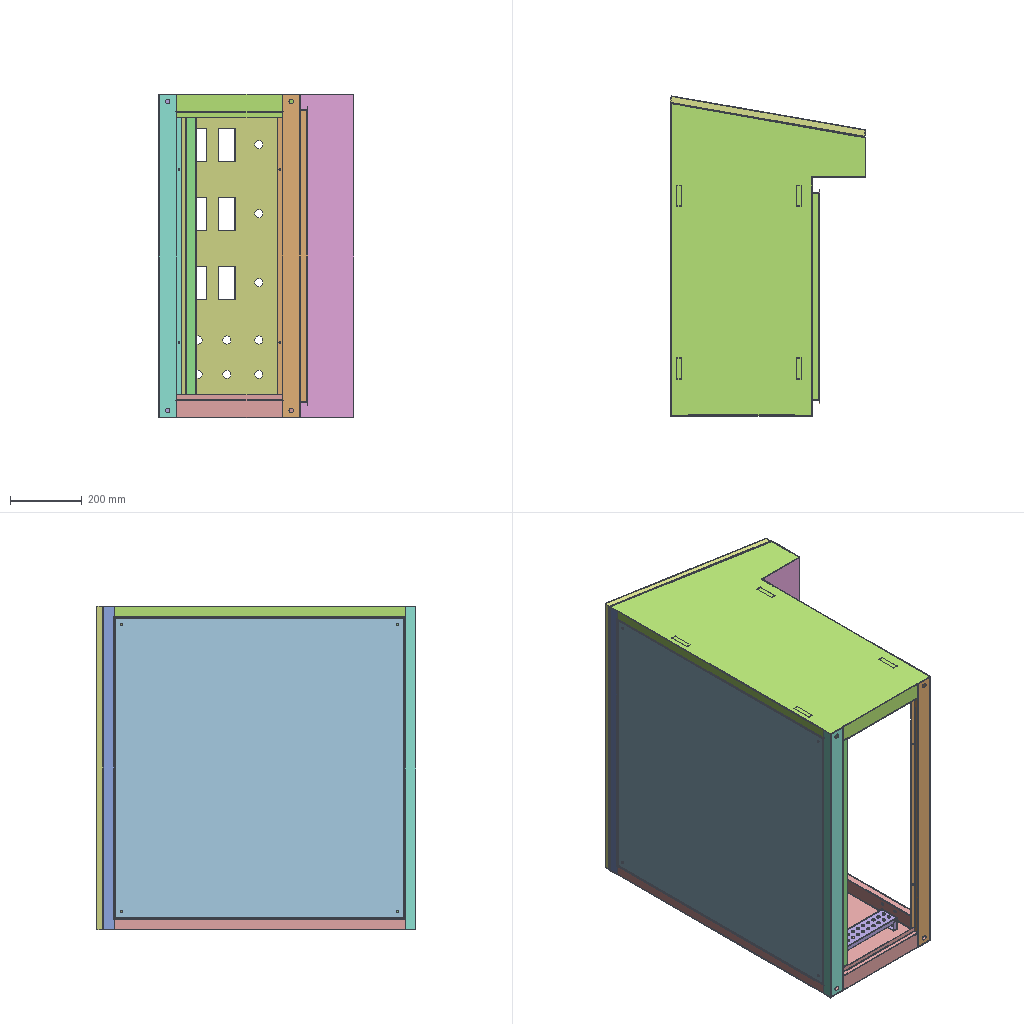Assembly | SolidWorks | 20 different items | 26 placed | box 545 x 890 x 900 mm
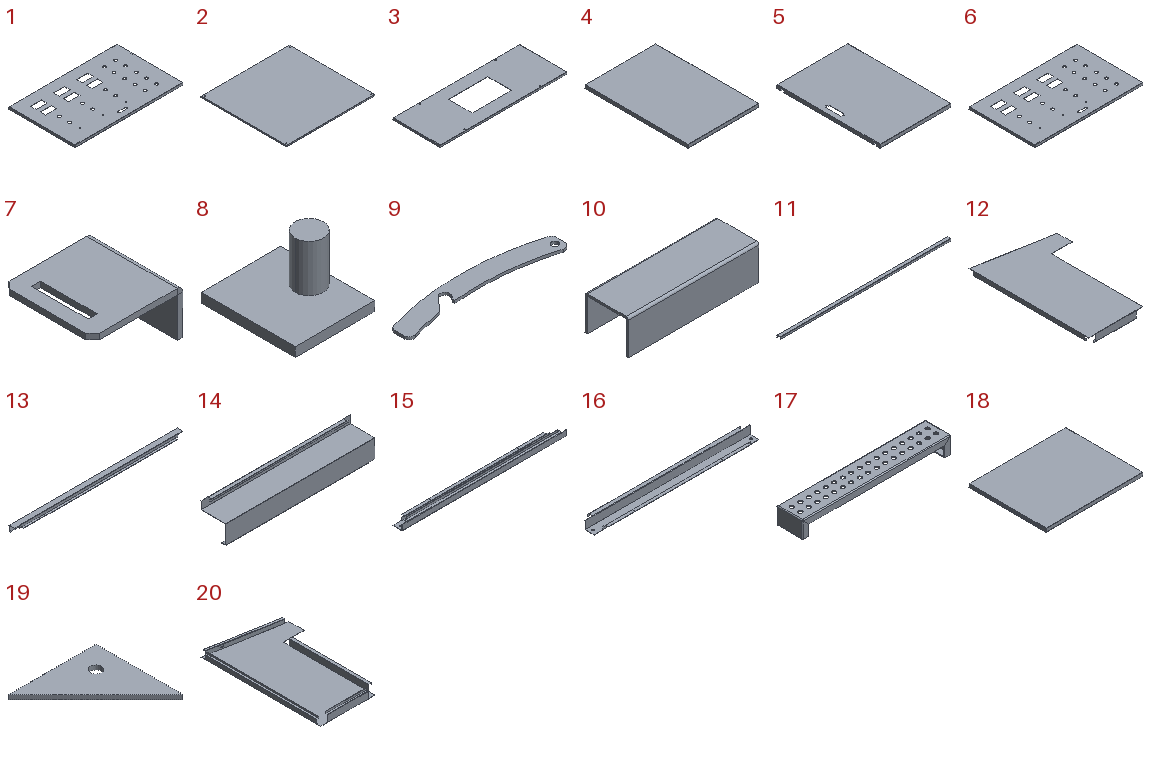Parts list (item | name | quantity | parent item | size | volume | features):
1 | (subassembly) | x1 | - | 900 x 550 x 20 mm | 806650 mm3 | -
2 | - | x1 | - | 837 x 807 x 13 mm | 1107218 mm3 | features EdgeFlange 2, FlatPattern 1, ICE 1, SMBaseFlange 1, SheetMetal 1
3 | - | x1 | - | 808 x 302 x 12 mm | 343087 mm3 | features ICE 2, EdgeFlange 1, FlatPattern 1, SMBaseFlange 1, SheetMetal 1
4 | - | x1 | - | 460.5 x 650 x 23.5 mm | 531757 mm3 | features EdgeFlange 4, FlatPattern 1, ICE 1, SMBaseFlange 1, SheetMetal 1
5 | - | x1 | - | 447 x 650 x 22 mm | 527115 mm3 | features ICE 3, EdgeFlange 2, FlatPattern 1, LPattern 1, SMBaseFlange 1, SheetMetal 1
6 | - | x1 | in 1 | 900 x 550 x 20 mm | 805688 mm3 | features EdgeFlange 2, ICE 2, FlatPattern 1, SMBaseFlange 1, SheetMetal 1
7 | - | x1 | - | 40 x 40 x 20 mm | 5420 mm3 | features Chamfer 1, EdgeFlange 1, FlatPattern 1, ICE 1, SMBaseFlange 1, SheetMetal 1
8 | - | x1 | in 1 | 17 x 20 x 12 mm | 962.743 mm3 | features FlatPattern 1, ICE 1, SMBaseFlange 1, SheetMetal 1
9 | - | x1 | - | 150 x 27.697 x 2.5 mm | 6095 mm3 | features Fillet 1, FlatPattern 1, ICE 1, SMBaseFlange 1, SheetMetal 1
10 | - | x1 | - | 90 x 30 x 24 mm | 10026 mm3 | features EdgeFlange 1, FlatPattern 1, SMBaseFlange 1, SheetMetal 1
11 | - | x1 | - | 950 x 20 x 12 mm | 74206 mm3 | features EdgeFlange 1, FlatPattern 1, SMBaseFlange 1, SheetMetal 1
12 | - | x1 | - | 543 x 881.04 x 63.5 mm | 714708 mm3 | features MirrorStock 1
13 | - | x1 | - | 897 x 52.929 x 32.409 mm | 134963 mm3 | features EdgeFlange 5, SMBaseFlange 2, FlatPattern 1, SheetMetal 1
14 | - | x1 | - | 897 x 150.5 x 176.459 mm | 509426 mm3 | features EdgeFlange 7, SMBaseFlange 3, FlatPattern 1, SheetMetal 1
15 | - | x1 | - | 897 x 63.5 x 40.5 mm | 164762 mm3 | features EdgeFlange 5, ICE 2, FlatPattern 1, SMBaseFlange 1, SheetMetal 1
16 | - | x1 | - | 897 x 84 x 45 mm | 190615 mm3 | features EdgeFlange 5, ICE 2, SMBaseFlange 2, FlatPattern 1, SheetMetal 1
17 | - | x4 | - | 350 x 60 x 40 mm | 69257 mm3 | features EdgeFlange 3, FlatPattern 1, ICE 1, SMBaseFlange 1, SheetMetal 1
18 | - | x1 | - | 816 x 650 x 30 mm | 1268651 mm3 | features EdgeFlange 2, FlatPattern 1, ICE 1, SMBaseFlange 1, SheetMetal 1
19 | - | x4 | - | 40 x 40 x 2 mm | 1559 mm3 | features FlatPattern 1, SMBaseFlange 1, SheetMetal 1
20 | - | x1 | - | 543 x 881.04 x 63.5 mm | 714708 mm3 | features EdgeFlange 12, ICE 4, FlatPattern 1, SMBaseFlange 1, SheetMetal 1
Mates (type | each side: item.copy, entity, surface, feature):
In the top assembly
Coincident | 20.1 face plane Edge-Flange1 | 13.1 face plane Base-Flange1
Coincident | 20.1 face plane Edge-Flange3 | 13.1 face plane Edge-Flange1
Coincident | 20.1 face plane Base-Flange1 | 13.1 face plane Edge-Flange1
Coincident | 13.1 face plane Edge-Flange1 | 12.1 face plane PAXX-425.001 Mirror
Coincident | 13.1 face plane Base-Flange1 | 12.1 face plane PAXX-425.001 Mirror | 2 times
Coincident | 12.1 face plane PAXX-425.001 Mirror | 14.1 face plane Base-Flange1 | 2 times
Coincident | 12.1 face plane PAXX-425.001 Mirror | 14.1 face plane Edge-Flange4
Coincident | 12.1 face plane PAXX-425.001 Mirror | 15.1 face plane Base-Flange1 | 2 times
Coincident | 12.1 face plane PAXX-425.001 Mirror | 15.1 face plane Edge-Flange1
Coincident | 12.1 face plane PAXX-425.001 Mirror | 16.1 face plane Edge-Flange1
Coincident | 12.1 face plane PAXX-425.001 Mirror | 16.1 face plane Base-Flange1 | 2 times
Coincident | 20.1 face plane Base-Flange1 | 17.1 face plane Edge-Flange3
Coincident | 20.1 face plane Edge-Flange4 | 17.1 face plane Edge-Flange1
Coincident | 12.1 face plane PAXX-425.001 Mirror | 17.2 face plane Edge-Flange3
Coincident | 17.1 face plane Edge-Flange2 | 17.2 face plane Edge-Flange2
Coincident | 17.1 face plane Edge-Flange1 | 17.2 face plane Edge-Flange1
DistanceDim | 17.1 face plane Edge-Flange2 | 20.1 face plane Edge-Flange10
DistanceDim | 18.1 face plane Edge-Flange1 | 17.1 face plane Base-Flange1
Concentric | 17.2 face cylinder Cut-Extrude1 | 18.1 face cylinder Cut-Extrude1 | 2 times
Coincident | 13.1 face plane Edge-Flange3 | 19.1 face plane Base-Flange1 | 2 times
Coincident | 12.1 face plane PAXX-425.001 Mirror | 19.1 face plane Base-Flange1
Coincident | 19.1 face plane Base-Flange1 | 19.2 face plane Base-Flange1
Coincident | 19.2 face plane Base-Flange1 | 19.3 face plane Base-Flange1
Coincident | 19.3 face plane Base-Flange1 | 19.4 face plane Base-Flange1
Coincident | 12.1 face plane PAXX-425.001 Mirror | 19.3 face plane Base-Flange1
Coincident | 15.1 face plane Edge-Flange3 | 19.3 face plane Base-Flange1
Coincident | 20.1 face plane Edge-Flange4 | 19.4 face plane Base-Flange1
Coincident | 13.1 face plane Edge-Flange3 | 19.4 face plane Base-Flange1
Coincident | 20.1 face plane Edge-Flange4 | 19.2 face plane Base-Flange1
Coincident | 15.1 face plane Edge-Flange3 | 19.2 face plane Base-Flange1
Coincident | 20.1 face plane Edge-Flange1 | 2.1 face plane Base-Flange1
DistanceDim | 2.1 face plane Edge-Flange1 | 20.1 face plane Edge-Flange2
DistanceDim | 2.1 face plane Edge-Flange1 | 13.1 face plane Edge-Flange2
Coincident | 20.1 face plane Base-Flange1 | 6.1 face plane Edge-Flange1
Coincident | 20.1 edge | 6.1 edge
Concentric | 8.1 face cylinder Boss-Extrude1 | 9.1 face cylinder Base-Flange1
Coincident | 8.1 face plane Base-Flange1 | 9.1 face plane Base-Flange1
In subassembly 1
Coincident | 6.2 face plane Edge-Flange2 | 8.2 face plane Base-Flange1
Coincident | 6.2 face plane Base-Flange1 | 8.2 face plane Base-Flange1
DistanceDim | 8.2 face plane Base-Flange1 | 6.2 face plane Edge-Flange1